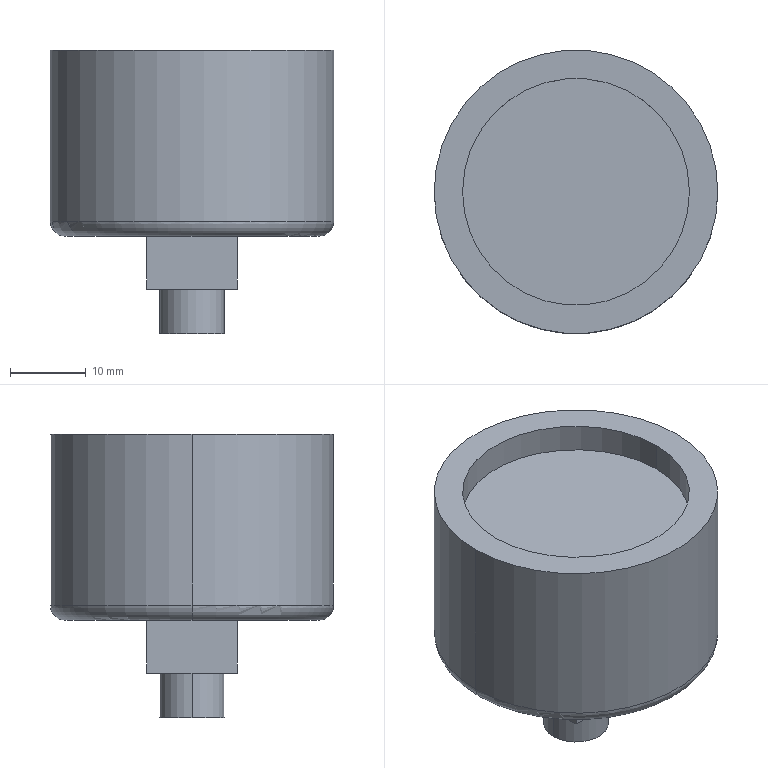Part | STEP file | AR20-G_GAUGE_HI | 1 solid | 17 faces | box 37.5 x 37.5 x 37.5 mm | volume 25733 mm3 | plane 9 | cylinder 6 | torus 2 | commonest cylinder face diameters 8.566 x2 30 x2 37.5 x2
STEP:
#1=CARTESIAN_POINT('',(0.,0.,0.));
#2=DIRECTION('',(0.,0.,1.));
#3=DIRECTION('',(1.,0.,0.));
#4=AXIS2_PLACEMENT_3D('',#1,#2,#3);
#5=CARTESIAN_POINT('',(4.283,0.,27.5));
#6=VERTEX_POINT('',#5);
#7=CARTESIAN_POINT('',(-4.283,0.,27.5));
#8=VERTEX_POINT('',#7);
#9=CARTESIAN_POINT('',(0.,0.,27.5));
#10=DIRECTION('',(0.,0.,1.));
#11=DIRECTION('',(1.,0.,0.));
#12=AXIS2_PLACEMENT_3D('',#9,#10,#11);
#13=CIRCLE('',#12,4.283);
#14=CARTESIAN_POINT('',(0.,0.,27.5));
#15=DIRECTION('',(0.,0.,1.));
#16=DIRECTION('',(1.,0.,0.));
#17=AXIS2_PLACEMENT_3D('',#14,#15,#16);
#18=CYLINDRICAL_SURFACE('',#17,4.283);
#19=CARTESIAN_POINT('',(0.,0.));
#20=DIRECTION('',(1.,0.));
#21=VECTOR('',#20,1.);
#22=LINE('',#19,#21);
#23=(GEOMETRIC_REPRESENTATION_CONTEXT(2)PARAMETRIC_REPRESENTATION_CONTEXT()REPRESENTATION_CONTEXT('',''));
#24=DEFINITIONAL_REPRESENTATION('',(#22),#23);
#25=PCURVE('',#18,#24);
#26=CARTESIAN_POINT('',(0.,4.283,27.5));
#27=DIRECTION('',(0.,0.,1.));
#28=DIRECTION('',(1.,0.,0.));
#29=AXIS2_PLACEMENT_3D('',#26,#27,#28);
#30=PLANE('',#29);
#31=CARTESIAN_POINT('',(0.,-4.283));
#32=DIRECTION('',(1.,0.));
#33=AXIS2_PLACEMENT_2D('',#31,#32);
#34=CIRCLE('',#33,4.283);
#35=(GEOMETRIC_REPRESENTATION_CONTEXT(2)PARAMETRIC_REPRESENTATION_CONTEXT()REPRESENTATION_CONTEXT('',''));
#36=DEFINITIONAL_REPRESENTATION('',(#34),#35);
#37=PCURVE('',#30,#36);
#38=SURFACE_CURVE('',#13,(#25,#37),.PCURVE_S1.);
#39=EDGE_CURVE('',#6,#8,#38,.T.);
#40=ORIENTED_EDGE('',*,*,#39,.T.);
#41=CARTESIAN_POINT('',(-4.283,0.,33.4));
#42=VERTEX_POINT('',#41);
#43=CARTESIAN_POINT('',(-4.283,0.,27.5));
#44=DIRECTION('',(0.,0.,1.));
#45=VECTOR('',#44,1.);
#46=LINE('',#43,#45);
#47=CARTESIAN_POINT('',(3.142,0.));
#48=DIRECTION('',(0.,1.));
#49=VECTOR('',#48,1.);
#50=LINE('',#47,#49);
#51=(GEOMETRIC_REPRESENTATION_CONTEXT(2)PARAMETRIC_REPRESENTATION_CONTEXT()REPRESENTATION_CONTEXT('',''));
#52=DEFINITIONAL_REPRESENTATION('',(#50),#51);
#53=PCURVE('',#18,#52);
#54=CARTESIAN_POINT('',(0.,0.,27.5));
#55=DIRECTION('',(0.,0.,1.));
#56=DIRECTION('',(1.,0.,0.));
#57=AXIS2_PLACEMENT_3D('',#54,#55,#56);
#58=CYLINDRICAL_SURFACE('',#57,4.283);
#59=CARTESIAN_POINT('',(3.142,0.));
#60=DIRECTION('',(0.,1.));
#61=VECTOR('',#60,1.);
#62=LINE('',#59,#61);
#63=(GEOMETRIC_REPRESENTATION_CONTEXT(2)PARAMETRIC_REPRESENTATION_CONTEXT()REPRESENTATION_CONTEXT('',''));
#64=DEFINITIONAL_REPRESENTATION('',(#62),#63);
#65=PCURVE('',#58,#64);
#66=SURFACE_CURVE('',#46,(#53,#65),.PCURVE_S1.);
#67=EDGE_CURVE('',#8,#42,#66,.T.);
#68=ORIENTED_EDGE('',*,*,#67,.T.);
#69=CARTESIAN_POINT('',(4.283,0.,33.4));
#70=VERTEX_POINT('',#69);
#71=CARTESIAN_POINT('',(0.,0.,33.4));
#72=DIRECTION('',(0.,0.,-1.));
#73=DIRECTION('',(1.,0.,0.));
#74=AXIS2_PLACEMENT_3D('',#71,#72,#73);
#75=CIRCLE('',#74,4.283);
#76=CARTESIAN_POINT('',(6.283,5.9));
#77=DIRECTION('',(-1.,0.));
#78=VECTOR('',#77,1.);
#79=LINE('',#76,#78);
#80=(GEOMETRIC_REPRESENTATION_CONTEXT(2)PARAMETRIC_REPRESENTATION_CONTEXT()REPRESENTATION_CONTEXT('',''));
#81=DEFINITIONAL_REPRESENTATION('',(#79),#80);
#82=PCURVE('',#18,#81);
#83=CARTESIAN_POINT('',(6.,-6.,33.4));
#84=DIRECTION('',(0.,0.,1.));
#85=DIRECTION('',(1.,0.,0.));
#86=AXIS2_PLACEMENT_3D('',#83,#84,#85);
#87=PLANE('',#86);
#88=CARTESIAN_POINT('',(-1.717,6.));
#89=CARTESIAN_POINT('',(-1.717,-1.418));
#90=CARTESIAN_POINT('',(-8.142,2.291));
#91=CARTESIAN_POINT('',(-14.566,6.));
#92=CARTESIAN_POINT('',(-8.142,9.709));
#93=CARTESIAN_POINT('',(-1.717,13.418));
#94=CARTESIAN_POINT('',(-1.717,6.));
#95=(BOUNDED_CURVE()B_SPLINE_CURVE(2,(#88,#89,#90,#91,#92,#93,#94),.UNSPECIFIED.,.T.,.F.)B_SPLINE_CURVE_WITH_KNOTS((1,2,2,2,2,1),(-2.094,0.,2.094,4.189,6.283,8.378),.UNSPECIFIED.)CURVE()GEOMETRIC_REPRESENTATION_ITEM()RATIONAL_B_SPLINE_CURVE((1.,0.5,1.,0.5,1.,0.5,1.))REPRESENTATION_ITEM(''));
#96=(GEOMETRIC_REPRESENTATION_CONTEXT(2)PARAMETRIC_REPRESENTATION_CONTEXT()REPRESENTATION_CONTEXT('',''));
#97=DEFINITIONAL_REPRESENTATION('',(#95),#96);
#98=PCURVE('',#87,#97);
#99=SURFACE_CURVE('',#75,(#82,#98),.PCURVE_S1.);
#100=EDGE_CURVE('',#42,#70,#99,.T.);
#101=ORIENTED_EDGE('',*,*,#100,.T.);
#102=CARTESIAN_POINT('',(4.283,0.,27.5));
#103=DIRECTION('',(0.,0.,1.));
#104=VECTOR('',#103,1.);
#105=LINE('',#102,#104);
#106=CARTESIAN_POINT('',(0.,0.));
#107=DIRECTION('',(0.,1.));
#108=VECTOR('',#107,1.);
#109=LINE('',#106,#108);
#110=(GEOMETRIC_REPRESENTATION_CONTEXT(2)PARAMETRIC_REPRESENTATION_CONTEXT()REPRESENTATION_CONTEXT('',''));
#111=DEFINITIONAL_REPRESENTATION('',(#109),#110);
#112=PCURVE('',#18,#111);
#113=CARTESIAN_POINT('',(6.283,0.));
#114=DIRECTION('',(0.,1.));
#115=VECTOR('',#114,1.);
#116=LINE('',#113,#115);
#117=(GEOMETRIC_REPRESENTATION_CONTEXT(2)PARAMETRIC_REPRESENTATION_CONTEXT()REPRESENTATION_CONTEXT('',''));
#118=DEFINITIONAL_REPRESENTATION('',(#116),#117);
#119=PCURVE('',#58,#118);
#120=SURFACE_CURVE('',#105,(#112,#119),.PCURVE_S1.);
#121=EDGE_CURVE('',#6,#70,#120,.T.);
#122=ORIENTED_EDGE('',*,*,#121,.F.);
#123=EDGE_LOOP('',(#40,#68,#101,#122));
#124=FACE_BOUND('',#123,.T.);
#125=ADVANCED_FACE('',(#124),#18,.T.);
#126=CARTESIAN_POINT('',(-15.,0.,65.));
#127=VERTEX_POINT('',#126);
#128=CARTESIAN_POINT('',(-15.,0.,61.2));
#129=VERTEX_POINT('',#128);
#130=CARTESIAN_POINT('',(-15.,0.,61.2));
#131=DIRECTION('',(0.,0.,-1.));
#132=VECTOR('',#131,1.);
#133=LINE('',#130,#132);
#134=CARTESIAN_POINT('',(0.,0.,61.2));
#135=DIRECTION('',(0.,0.,-1.));
#136=DIRECTION('',(-1.,0.,0.));
#137=AXIS2_PLACEMENT_3D('',#134,#135,#136);
#138=CYLINDRICAL_SURFACE('',#137,15.);
#139=CARTESIAN_POINT('',(6.283,0.));
#140=DIRECTION('',(0.,1.));
#141=VECTOR('',#140,1.);
#142=LINE('',#139,#141);
#143=(GEOMETRIC_REPRESENTATION_CONTEXT(2)PARAMETRIC_REPRESENTATION_CONTEXT()REPRESENTATION_CONTEXT('',''));
#144=DEFINITIONAL_REPRESENTATION('',(#142),#143);
#145=PCURVE('',#138,#144);
#146=CARTESIAN_POINT('',(0.,0.,61.2));
#147=DIRECTION('',(0.,0.,-1.));
#148=DIRECTION('',(-1.,0.,0.));
#149=AXIS2_PLACEMENT_3D('',#146,#147,#148);
#150=CYLINDRICAL_SURFACE('',#149,15.);
#151=CARTESIAN_POINT('',(0.,0.));
#152=DIRECTION('',(0.,1.));
#153=VECTOR('',#152,1.);
#154=LINE('',#151,#153);
#155=(GEOMETRIC_REPRESENTATION_CONTEXT(2)PARAMETRIC_REPRESENTATION_CONTEXT()REPRESENTATION_CONTEXT('',''));
#156=DEFINITIONAL_REPRESENTATION('',(#154),#155);
#157=PCURVE('',#150,#156);
#158=SURFACE_CURVE('',#133,(#145,#157),.PCURVE_S1.);
#159=EDGE_CURVE('',#127,#129,#158,.T.);
#160=ORIENTED_EDGE('',*,*,#159,.T.);
#161=CARTESIAN_POINT('',(15.,0.,61.2));
#162=VERTEX_POINT('',#161);
#163=CARTESIAN_POINT('',(0.,0.,61.2));
#164=DIRECTION('',(0.,0.,-1.));
#165=DIRECTION('',(-1.,0.,0.));
#166=AXIS2_PLACEMENT_3D('',#163,#164,#165);
#167=CIRCLE('',#166,15.);
#168=CARTESIAN_POINT('',(0.,0.));
#169=DIRECTION('',(1.,0.));
#170=VECTOR('',#169,1.);
#171=LINE('',#168,#170);
#172=(GEOMETRIC_REPRESENTATION_CONTEXT(2)PARAMETRIC_REPRESENTATION_CONTEXT()REPRESENTATION_CONTEXT('',''));
#173=DEFINITIONAL_REPRESENTATION('',(#171),#172);
#174=PCURVE('',#138,#173);
#175=CARTESIAN_POINT('',(0.,-15.,61.2));
#176=DIRECTION('',(0.,0.,-1.));
#177=DIRECTION('',(-1.,0.,0.));
#178=AXIS2_PLACEMENT_3D('',#175,#176,#177);
#179=PLANE('',#178);
#180=CARTESIAN_POINT('',(0.,15.));
#181=DIRECTION('',(1.,0.));
#182=AXIS2_PLACEMENT_2D('',#180,#181);
#183=CIRCLE('',#182,15.);
#184=(GEOMETRIC_REPRESENTATION_CONTEXT(2)PARAMETRIC_REPRESENTATION_CONTEXT()REPRESENTATION_CONTEXT('',''));
#185=DEFINITIONAL_REPRESENTATION('',(#183),#184);
#186=PCURVE('',#179,#185);
#187=SURFACE_CURVE('',#167,(#174,#186),.PCURVE_S1.);
#188=EDGE_CURVE('',#162,#129,#187,.T.);
#189=ORIENTED_EDGE('',*,*,#188,.F.);
#190=CARTESIAN_POINT('',(15.,0.,65.));
#191=VERTEX_POINT('',#190);
#192=CARTESIAN_POINT('',(15.,0.,61.2));
#193=DIRECTION('',(0.,0.,-1.));
#194=VECTOR('',#193,1.);
#195=LINE('',#192,#194);
#196=CARTESIAN_POINT('',(3.142,0.));
#197=DIRECTION('',(0.,1.));
#198=VECTOR('',#197,1.);
#199=LINE('',#196,#198);
#200=(GEOMETRIC_REPRESENTATION_CONTEXT(2)PARAMETRIC_REPRESENTATION_CONTEXT()REPRESENTATION_CONTEXT('',''));
#201=DEFINITIONAL_REPRESENTATION('',(#199),#200);
#202=PCURVE('',#138,#201);
#203=CARTESIAN_POINT('',(3.142,0.));
#204=DIRECTION('',(0.,1.));
#205=VECTOR('',#204,1.);
#206=LINE('',#203,#205);
#207=(GEOMETRIC_REPRESENTATION_CONTEXT(2)PARAMETRIC_REPRESENTATION_CONTEXT()REPRESENTATION_CONTEXT('',''));
#208=DEFINITIONAL_REPRESENTATION('',(#206),#207);
#209=PCURVE('',#150,#208);
#210=SURFACE_CURVE('',#195,(#202,#209),.PCURVE_S1.);
#211=EDGE_CURVE('',#191,#162,#210,.T.);
#212=ORIENTED_EDGE('',*,*,#211,.F.);
#213=CARTESIAN_POINT('',(0.,0.,65.));
#214=DIRECTION('',(0.,0.,-1.));
#215=DIRECTION('',(-1.,0.,0.));
#216=AXIS2_PLACEMENT_3D('',#213,#214,#215);
#217=CIRCLE('',#216,15.);
#218=CARTESIAN_POINT('',(0.,-3.8));
#219=DIRECTION('',(1.,0.));
#220=VECTOR('',#219,1.);
#221=LINE('',#218,#220);
#222=(GEOMETRIC_REPRESENTATION_CONTEXT(2)PARAMETRIC_REPRESENTATION_CONTEXT()REPRESENTATION_CONTEXT('',''));
#223=DEFINITIONAL_REPRESENTATION('',(#221),#222);
#224=PCURVE('',#138,#223);
#225=CARTESIAN_POINT('',(0.,-18.75,65.));
#226=DIRECTION('',(0.,0.,-1.));
#227=DIRECTION('',(-1.,0.,0.));
#228=AXIS2_PLACEMENT_3D('',#225,#226,#227);
#229=PLANE('',#228);
#230=CARTESIAN_POINT('',(0.,18.75));
#231=DIRECTION('',(1.,0.));
#232=AXIS2_PLACEMENT_2D('',#230,#231);
#233=CIRCLE('',#232,15.);
#234=(GEOMETRIC_REPRESENTATION_CONTEXT(2)PARAMETRIC_REPRESENTATION_CONTEXT()REPRESENTATION_CONTEXT('',''));
#235=DEFINITIONAL_REPRESENTATION('',(#233),#234);
#236=PCURVE('',#229,#235);
#237=SURFACE_CURVE('',#217,(#224,#236),.PCURVE_S1.);
#238=EDGE_CURVE('',#191,#127,#237,.T.);
#239=ORIENTED_EDGE('',*,*,#238,.T.);
#240=EDGE_LOOP('',(#160,#189,#212,#239));
#241=FACE_BOUND('',#240,.F.);
#242=ADVANCED_FACE('',(#241),#138,.F.);
#243=CARTESIAN_POINT('',(-18.75,0.,65.));
#244=VERTEX_POINT('',#243);
#245=CARTESIAN_POINT('',(18.75,0.,65.));
#246=VERTEX_POINT('',#245);
#247=CARTESIAN_POINT('',(0.,0.,65.));
#248=DIRECTION('',(0.,0.,-1.));
#249=DIRECTION('',(-1.,0.,0.));
#250=AXIS2_PLACEMENT_3D('',#247,#248,#249);
#251=CIRCLE('',#250,18.75);
#252=CARTESIAN_POINT('',(0.,0.,61.2));
#253=DIRECTION('',(0.,0.,-1.));
#254=DIRECTION('',(-1.,0.,0.));
#255=AXIS2_PLACEMENT_3D('',#252,#253,#254);
#256=CYLINDRICAL_SURFACE('',#255,18.75);
#257=CARTESIAN_POINT('',(0.,-3.8));
#258=DIRECTION('',(1.,0.));
#259=VECTOR('',#258,1.);
#260=LINE('',#257,#259);
#261=(GEOMETRIC_REPRESENTATION_CONTEXT(2)PARAMETRIC_REPRESENTATION_CONTEXT()REPRESENTATION_CONTEXT('',''));
#262=DEFINITIONAL_REPRESENTATION('',(#260),#261);
#263=PCURVE('',#256,#262);
#264=CARTESIAN_POINT('',(0.,18.75));
#265=DIRECTION('',(1.,0.));
#266=AXIS2_PLACEMENT_2D('',#264,#265);
#267=CIRCLE('',#266,18.75);
#268=(GEOMETRIC_REPRESENTATION_CONTEXT(2)PARAMETRIC_REPRESENTATION_CONTEXT()REPRESENTATION_CONTEXT('',''));
#269=DEFINITIONAL_REPRESENTATION('',(#267),#268);
#270=PCURVE('',#229,#269);
#271=SURFACE_CURVE('',#251,(#263,#270),.PCURVE_S1.);
#272=EDGE_CURVE('',#244,#246,#271,.T.);
#273=ORIENTED_EDGE('',*,*,#272,.T.);
#274=CARTESIAN_POINT('',(18.75,0.,42.4));
#275=VERTEX_POINT('',#274);
#276=CARTESIAN_POINT('',(18.75,0.,61.2));
#277=DIRECTION('',(0.,0.,-1.));
#278=VECTOR('',#277,1.);
#279=LINE('',#276,#278);
#280=CARTESIAN_POINT('',(3.142,0.));
#281=DIRECTION('',(0.,1.));
#282=VECTOR('',#281,1.);
#283=LINE('',#280,#282);
#284=(GEOMETRIC_REPRESENTATION_CONTEXT(2)PARAMETRIC_REPRESENTATION_CONTEXT()REPRESENTATION_CONTEXT('',''));
#285=DEFINITIONAL_REPRESENTATION('',(#283),#284);
#286=PCURVE('',#256,#285);
#287=CARTESIAN_POINT('',(0.,0.,61.2));
#288=DIRECTION('',(0.,0.,-1.));
#289=DIRECTION('',(-1.,0.,0.));
#290=AXIS2_PLACEMENT_3D('',#287,#288,#289);
#291=CYLINDRICAL_SURFACE('',#290,18.75);
#292=CARTESIAN_POINT('',(3.142,0.));
#293=DIRECTION('',(0.,1.));
#294=VECTOR('',#293,1.);
#295=LINE('',#292,#294);
#296=(GEOMETRIC_REPRESENTATION_CONTEXT(2)PARAMETRIC_REPRESENTATION_CONTEXT()REPRESENTATION_CONTEXT('',''));
#297=DEFINITIONAL_REPRESENTATION('',(#295),#296);
#298=PCURVE('',#291,#297);
#299=SURFACE_CURVE('',#279,(#286,#298),.PCURVE_S1.);
#300=EDGE_CURVE('',#246,#275,#299,.T.);
#301=ORIENTED_EDGE('',*,*,#300,.T.);
#302=CARTESIAN_POINT('',(-18.75,0.,42.4));
#303=VERTEX_POINT('',#302);
#304=CARTESIAN_POINT('',(0.,0.,42.4));
#305=DIRECTION('',(0.,0.,-1.));
#306=DIRECTION('',(-1.,0.,0.));
#307=AXIS2_PLACEMENT_3D('',#304,#305,#306);
#308=CIRCLE('',#307,18.75);
#309=CARTESIAN_POINT('',(0.,18.8));
#310=DIRECTION('',(1.,0.));
#311=VECTOR('',#310,1.);
#312=LINE('',#309,#311);
#313=(GEOMETRIC_REPRESENTATION_CONTEXT(2)PARAMETRIC_REPRESENTATION_CONTEXT()REPRESENTATION_CONTEXT('',''));
#314=DEFINITIONAL_REPRESENTATION('',(#312),#313);
#315=PCURVE('',#256,#314);
#316=CARTESIAN_POINT('',(0.,0.,42.4));
#317=DIRECTION('',(0.,0.,-1.));
#318=DIRECTION('',(-1.,0.,0.));
#319=AXIS2_PLACEMENT_3D('',#316,#317,#318);
#320=TOROIDAL_SURFACE('',#319,16.75,2.);
#321=CARTESIAN_POINT('',(0.,0.));
#322=DIRECTION('',(1.,0.));
#323=VECTOR('',#322,1.);
#324=LINE('',#321,#323);
#325=(GEOMETRIC_REPRESENTATION_CONTEXT(2)PARAMETRIC_REPRESENTATION_CONTEXT()REPRESENTATION_CONTEXT('',''));
#326=DEFINITIONAL_REPRESENTATION('',(#324),#325);
#327=PCURVE('',#320,#326);
#328=SURFACE_CURVE('',#308,(#315,#327),.PCURVE_S1.);
#329=EDGE_CURVE('',#303,#275,#328,.T.);
#330=ORIENTED_EDGE('',*,*,#329,.F.);
#331=CARTESIAN_POINT('',(-18.75,0.,61.2));
#332=DIRECTION('',(0.,0.,-1.));
#333=VECTOR('',#332,1.);
#334=LINE('',#331,#333);
#335=CARTESIAN_POINT('',(0.,0.));
#336=DIRECTION('',(0.,1.));
#337=VECTOR('',#336,1.);
#338=LINE('',#335,#337);
#339=(GEOMETRIC_REPRESENTATION_CONTEXT(2)PARAMETRIC_REPRESENTATION_CONTEXT()REPRESENTATION_CONTEXT('',''));
#340=DEFINITIONAL_REPRESENTATION('',(#338),#339);
#341=PCURVE('',#256,#340);
#342=CARTESIAN_POINT('',(6.283,0.));
#343=DIRECTION('',(0.,1.));
#344=VECTOR('',#343,1.);
#345=LINE('',#342,#344);
#346=(GEOMETRIC_REPRESENTATION_CONTEXT(2)PARAMETRIC_REPRESENTATION_CONTEXT()REPRESENTATION_CONTEXT('',''));
#347=DEFINITIONAL_REPRESENTATION('',(#345),#346);
#348=PCURVE('',#291,#347);
#349=SURFACE_CURVE('',#334,(#341,#348),.PCURVE_S1.);
#350=EDGE_CURVE('',#244,#303,#349,.T.);
#351=ORIENTED_EDGE('',*,*,#350,.F.);
#352=EDGE_LOOP('',(#273,#301,#330,#351));
#353=FACE_BOUND('',#352,.T.);
#354=ADVANCED_FACE('',(#353),#256,.T.);
#355=ORIENTED_EDGE('',*,*,#329,.T.);
#356=CARTESIAN_POINT('',(16.75,0.,40.4));
#357=VERTEX_POINT('',#356);
#358=CARTESIAN_POINT('',(16.75,0.,42.4));
#359=DIRECTION('',(0.,1.,0.));
#360=DIRECTION('',(-1.,0.,0.));
#361=AXIS2_PLACEMENT_3D('',#358,#359,#360);
#362=CIRCLE('',#361,2.);
#363=CARTESIAN_POINT('',(3.142,-3.142));
#364=DIRECTION('',(0.,1.));
#365=VECTOR('',#364,1.);
#366=LINE('',#363,#365);
#367=(GEOMETRIC_REPRESENTATION_CONTEXT(2)PARAMETRIC_REPRESENTATION_CONTEXT()REPRESENTATION_CONTEXT('',''));
#368=DEFINITIONAL_REPRESENTATION('',(#366),#367);
#369=PCURVE('',#320,#368);
#370=CARTESIAN_POINT('',(0.,0.,42.4));
#371=DIRECTION('',(0.,0.,-1.));
#372=DIRECTION('',(-1.,0.,0.));
#373=AXIS2_PLACEMENT_3D('',#370,#371,#372);
#374=TOROIDAL_SURFACE('',#373,16.75,2.);
#375=CARTESIAN_POINT('',(3.142,-3.142));
#376=DIRECTION('',(0.,1.));
#377=VECTOR('',#376,1.);
#378=LINE('',#375,#377);
#379=(GEOMETRIC_REPRESENTATION_CONTEXT(2)PARAMETRIC_REPRESENTATION_CONTEXT()REPRESENTATION_CONTEXT('',''));
#380=DEFINITIONAL_REPRESENTATION('',(#378),#379);
#381=PCURVE('',#374,#380);
#382=SURFACE_CURVE('',#362,(#369,#381),.PCURVE_S1.);
#383=EDGE_CURVE('',#275,#357,#382,.T.);
#384=ORIENTED_EDGE('',*,*,#383,.T.);
#385=CARTESIAN_POINT('',(-16.75,0.,40.4));
#386=VERTEX_POINT('',#385);
#387=CARTESIAN_POINT('',(0.,0.,40.4));
#388=DIRECTION('',(0.,0.,-1.));
#389=DIRECTION('',(-1.,0.,0.));
#390=AXIS2_PLACEMENT_3D('',#387,#388,#389);
#391=CIRCLE('',#390,16.75);
#392=CARTESIAN_POINT('',(0.,1.571));
#393=DIRECTION('',(1.,0.));
#394=VECTOR('',#393,1.);
#395=LINE('',#392,#394);
#396=(GEOMETRIC_REPRESENTATION_CONTEXT(2)PARAMETRIC_REPRESENTATION_CONTEXT()REPRESENTATION_CONTEXT('',''));
#397=DEFINITIONAL_REPRESENTATION('',(#395),#396);
#398=PCURVE('',#320,#397);
#399=CARTESIAN_POINT('',(0.,0.,40.4));
#400=DIRECTION('',(0.,0.,1.));
#401=DIRECTION('',(1.,0.,0.));
#402=AXIS2_PLACEMENT_3D('',#399,#400,#401);
#403=PLANE('',#402);
#404=CARTESIAN_POINT('',(-16.75,0.));
#405=CARTESIAN_POINT('',(-16.75,29.012));
#406=CARTESIAN_POINT('',(8.375,14.506));
#407=CARTESIAN_POINT('',(33.5,0.));
#408=CARTESIAN_POINT('',(8.375,-14.506));
#409=CARTESIAN_POINT('',(-16.75,-29.012));
#410=CARTESIAN_POINT('',(-16.75,0.));
#411=(BOUNDED_CURVE()B_SPLINE_CURVE(2,(#404,#405,#406,#407,#408,#409,#410),.UNSPECIFIED.,.T.,.F.)B_SPLINE_CURVE_WITH_KNOTS((1,2,2,2,2,1),(-2.094,0.,2.094,4.189,6.283,8.378),.UNSPECIFIED.)CURVE()GEOMETRIC_REPRESENTATION_ITEM()RATIONAL_B_SPLINE_CURVE((1.,0.5,1.,0.5,1.,0.5,1.))REPRESENTATION_ITEM(''));
#412=(GEOMETRIC_REPRESENTATION_CONTEXT(2)PARAMETRIC_REPRESENTATION_CONTEXT()REPRESENTATION_CONTEXT('',''));
#413=DEFINITIONAL_REPRESENTATION('',(#411),#412);
#414=PCURVE('',#403,#413);
#415=SURFACE_CURVE('',#391,(#398,#414),.PCURVE_S1.);
#416=EDGE_CURVE('',#386,#357,#415,.T.);
#417=ORIENTED_EDGE('',*,*,#416,.F.);
#418=CARTESIAN_POINT('',(-16.75,0.,42.4));
#419=DIRECTION('',(0.,-1.,0.));
#420=DIRECTION('',(0.,0.,-1.));
#421=AXIS2_PLACEMENT_3D('',#418,#419,#420);
#422=CIRCLE('',#421,2.);
#423=CARTESIAN_POINT('',(0.,-4.712));
#424=DIRECTION('',(0.,1.));
#425=VECTOR('',#424,1.);
#426=LINE('',#423,#425);
#427=(GEOMETRIC_REPRESENTATION_CONTEXT(2)PARAMETRIC_REPRESENTATION_CONTEXT()REPRESENTATION_CONTEXT('',''));
#428=DEFINITIONAL_REPRESENTATION('',(#426),#427);
#429=PCURVE('',#320,#428);
#430=CARTESIAN_POINT('',(6.283,-4.712));
#431=DIRECTION('',(0.,1.));
#432=VECTOR('',#431,1.);
#433=LINE('',#430,#432);
#434=(GEOMETRIC_REPRESENTATION_CONTEXT(2)PARAMETRIC_REPRESENTATION_CONTEXT()REPRESENTATION_CONTEXT('',''));
#435=DEFINITIONAL_REPRESENTATION('',(#433),#434);
#436=PCURVE('',#374,#435);
#437=SURFACE_CURVE('',#422,(#429,#436),.PCURVE_S1.);
#438=EDGE_CURVE('',#303,#386,#437,.T.);
#439=ORIENTED_EDGE('',*,*,#438,.F.);
#440=EDGE_LOOP('',(#355,#384,#417,#439));
#441=FACE_BOUND('',#440,.T.);
#442=ADVANCED_FACE('',(#441),#320,.T.);
#443=CARTESIAN_POINT('',(6.,-6.,33.4));
#444=VERTEX_POINT('',#443);
#445=CARTESIAN_POINT('',(-6.,-6.,33.4));
#446=VERTEX_POINT('',#445);
#447=CARTESIAN_POINT('',(6.,-6.,33.4));
#448=DIRECTION('',(-1.,0.,0.));
#449=VECTOR('',#448,1.);
#450=LINE('',#447,#449);
#451=CARTESIAN_POINT('',(0.,0.));
#452=DIRECTION('',(-1.,0.));
#453=VECTOR('',#452,1.);
#454=LINE('',#451,#453);
#455=(GEOMETRIC_REPRESENTATION_CONTEXT(2)PARAMETRIC_REPRESENTATION_CONTEXT()REPRESENTATION_CONTEXT('',''));
#456=DEFINITIONAL_REPRESENTATION('',(#454),#455);
#457=PCURVE('',#87,#456);
#458=CARTESIAN_POINT('',(6.,-6.,40.4));
#459=DIRECTION('',(0.,1.,0.));
#460=DIRECTION('',(0.,0.,1.));
#461=AXIS2_PLACEMENT_3D('',#458,#459,#460);
#462=PLANE('',#461);
#463=CARTESIAN_POINT('',(-7.,0.));
#464=DIRECTION('',(0.,-1.));
#465=VECTOR('',#464,1.);
#466=LINE('',#463,#465);
#467=(GEOMETRIC_REPRESENTATION_CONTEXT(2)PARAMETRIC_REPRESENTATION_CONTEXT()REPRESENTATION_CONTEXT('',''));
#468=DEFINITIONAL_REPRESENTATION('',(#466),#467);
#469=PCURVE('',#462,#468);
#470=SURFACE_CURVE('',#450,(#457,#469),.PCURVE_S1.);
#471=EDGE_CURVE('',#444,#446,#470,.T.);
#472=ORIENTED_EDGE('',*,*,#471,.T.);
#473=CARTESIAN_POINT('',(-6.,6.,33.4));
#474=VERTEX_POINT('',#473);
#475=CARTESIAN_POINT('',(-6.,-6.,33.4));
#476=DIRECTION('',(0.,1.,0.));
#477=VECTOR('',#476,1.);
#478=LINE('',#475,#477);
#479=CARTESIAN_POINT('',(-12.,0.));
#480=DIRECTION('',(0.,1.));
#481=VECTOR('',#480,1.);
#482=LINE('',#479,#481);
#483=(GEOMETRIC_REPRESENTATION_CONTEXT(2)PARAMETRIC_REPRESENTATION_CONTEXT()REPRESENTATION_CONTEXT('',''));
#484=DEFINITIONAL_REPRESENTATION('',(#482),#483);
#485=PCURVE('',#87,#484);
#486=CARTESIAN_POINT('',(-6.,0.,0.));
#487=DIRECTION('',(1.,0.,0.));
#488=DIRECTION('',(0.,0.,-1.));
#489=AXIS2_PLACEMENT_3D('',#486,#487,#488);
#490=PLANE('',#489);
#491=CARTESIAN_POINT('',(-33.4,-6.));
#492=DIRECTION('',(0.,1.));
#493=VECTOR('',#492,1.);
#494=LINE('',#491,#493);
#495=(GEOMETRIC_REPRESENTATION_CONTEXT(2)PARAMETRIC_REPRESENTATION_CONTEXT()REPRESENTATION_CONTEXT('',''));
#496=DEFINITIONAL_REPRESENTATION('',(#494),#495);
#497=PCURVE('',#490,#496);
#498=SURFACE_CURVE('',#478,(#485,#497),.PCURVE_S1.);
#499=EDGE_CURVE('',#446,#474,#498,.T.);
#500=ORIENTED_EDGE('',*,*,#499,.T.);
#501=CARTESIAN_POINT('',(6.,6.,33.4));
#502=VERTEX_POINT('',#501);
#503=CARTESIAN_POINT('',(6.,6.,33.4));
#504=DIRECTION('',(-1.,0.,0.));
#505=VECTOR('',#504,1.);
#506=LINE('',#503,#505);
#507=CARTESIAN_POINT('',(0.,12.));
#508=DIRECTION('',(-1.,0.));
#509=VECTOR('',#508,1.);
#510=LINE('',#507,#509);
#511=(GEOMETRIC_REPRESENTATION_CONTEXT(2)PARAMETRIC_REPRESENTATION_CONTEXT()REPRESENTATION_CONTEXT('',''));
#512=DEFINITIONAL_REPRESENTATION('',(#510),#511);
#513=PCURVE('',#87,#512);
#514=CARTESIAN_POINT('',(6.,6.,33.4));
#515=DIRECTION('',(0.,-1.,0.));
#516=DIRECTION('',(0.,0.,-1.));
#517=AXIS2_PLACEMENT_3D('',#514,#515,#516);
#518=PLANE('',#517);
#519=CARTESIAN_POINT('',(0.,0.));
#520=DIRECTION('',(0.,-1.));
#521=VECTOR('',#520,1.);
#522=LINE('',#519,#521);
#523=(GEOMETRIC_REPRESENTATION_CONTEXT(2)PARAMETRIC_REPRESENTATION_CONTEXT()REPRESENTATION_CONTEXT('',''));
#524=DEFINITIONAL_REPRESENTATION('',(#522),#523);
#525=PCURVE('',#518,#524);
#526=SURFACE_CURVE('',#506,(#513,#525),.PCURVE_S1.);
#527=EDGE_CURVE('',#502,#474,#526,.T.);
#528=ORIENTED_EDGE('',*,*,#527,.F.);
#529=CARTESIAN_POINT('',(6.,-6.,33.4));
#530=DIRECTION('',(0.,1.,0.));
#531=VECTOR('',#530,1.);
#532=LINE('',#529,#531);
#533=CARTESIAN_POINT('',(0.,0.));
#534=DIRECTION('',(0.,1.));
#535=VECTOR('',#534,1.);
#536=LINE('',#533,#535);
#537=(GEOMETRIC_REPRESENTATION_CONTEXT(2)PARAMETRIC_REPRESENTATION_CONTEXT()REPRESENTATION_CONTEXT('',''));
#538=DEFINITIONAL_REPRESENTATION('',(#536),#537);
#539=PCURVE('',#87,#538);
#540=CARTESIAN_POINT('',(6.,0.,0.));
#541=DIRECTION('',(1.,0.,0.));
#542=DIRECTION('',(0.,0.,-1.));
#543=AXIS2_PLACEMENT_3D('',#540,#541,#542);
#544=PLANE('',#543);
#545=CARTESIAN_POINT('',(-33.4,-6.));
#546=DIRECTION('',(0.,1.));
#547=VECTOR('',#546,1.);
#548=LINE('',#545,#547);
#549=(GEOMETRIC_REPRESENTATION_CONTEXT(2)PARAMETRIC_REPRESENTATION_CONTEXT()REPRESENTATION_CONTEXT('',''));
#550=DEFINITIONAL_REPRESENTATION('',(#548),#549);
#551=PCURVE('',#544,#550);
#552=SURFACE_CURVE('',#532,(#539,#551),.PCURVE_S1.);
#553=EDGE_CURVE('',#444,#502,#552,.T.);
#554=ORIENTED_EDGE('',*,*,#553,.F.);
#555=EDGE_LOOP('',(#472,#500,#528,#554));
#556=FACE_BOUND('',#555,.T.);
#557=CARTESIAN_POINT('',(0.,0.,33.4));
#558=DIRECTION('',(0.,0.,-1.));
#559=DIRECTION('',(1.,0.,0.));
#560=AXIS2_PLACEMENT_3D('',#557,#558,#559);
#561=CIRCLE('',#560,4.283);
#562=CARTESIAN_POINT('',(-1.717,6.));
#563=CARTESIAN_POINT('',(-1.717,-1.418));
#564=CARTESIAN_POINT('',(-8.142,2.291));
#565=CARTESIAN_POINT('',(-14.566,6.));
#566=CARTESIAN_POINT('',(-8.142,9.709));
#567=CARTESIAN_POINT('',(-1.717,13.418));
#568=CARTESIAN_POINT('',(-1.717,6.));
#569=(BOUNDED_CURVE()B_SPLINE_CURVE(2,(#562,#563,#564,#565,#566,#567,#568),.UNSPECIFIED.,.T.,.F.)B_SPLINE_CURVE_WITH_KNOTS((1,2,2,2,2,1),(-2.094,0.,2.094,4.189,6.283,8.378),.UNSPECIFIED.)CURVE()GEOMETRIC_REPRESENTATION_ITEM()RATIONAL_B_SPLINE_CURVE((1.,0.5,1.,0.5,1.,0.5,1.))REPRESENTATION_ITEM(''));
#570=(GEOMETRIC_REPRESENTATION_CONTEXT(2)PARAMETRIC_REPRESENTATION_CONTEXT()REPRESENTATION_CONTEXT('',''));
#571=DEFINITIONAL_REPRESENTATION('',(#569),#570);
#572=PCURVE('',#87,#571);
#573=CARTESIAN_POINT('',(6.283,5.9));
#574=DIRECTION('',(-1.,0.));
#575=VECTOR('',#574,1.);
#576=LINE('',#573,#575);
#577=(GEOMETRIC_REPRESENTATION_CONTEXT(2)PARAMETRIC_REPRESENTATION_CONTEXT()REPRESENTATION_CONTEXT('',''));
#578=DEFINITIONAL_REPRESENTATION('',(#576),#577);
#579=PCURVE('',#58,#578);
#580=SURFACE_CURVE('',#561,(#572,#579),.PCURVE_S1.);
#581=EDGE_CURVE('',#70,#42,#580,.T.);
#582=ORIENTED_EDGE('',*,*,#581,.F.);
#583=ORIENTED_EDGE('',*,*,#100,.F.);
#584=EDGE_LOOP('',(#582,#583));
#585=FACE_BOUND('',#584,.T.);
#586=ADVANCED_FACE('',(#556,#585),#87,.F.);
#587=CARTESIAN_POINT('',(6.,-6.,40.4));
#588=VERTEX_POINT('',#587);
#589=CARTESIAN_POINT('',(-6.,-6.,40.4));
#590=VERTEX_POINT('',#589);
#591=CARTESIAN_POINT('',(6.,-6.,40.4));
#592=DIRECTION('',(-1.,0.,0.));
#593=VECTOR('',#592,1.);
#594=LINE('',#591,#593);
#595=CARTESIAN_POINT('',(6.,-6.));
#596=DIRECTION('',(-1.,0.));
#597=VECTOR('',#596,1.);
#598=LINE('',#595,#597);
#599=(GEOMETRIC_REPRESENTATION_CONTEXT(2)PARAMETRIC_REPRESENTATION_CONTEXT()REPRESENTATION_CONTEXT('',''));
#600=DEFINITIONAL_REPRESENTATION('',(#598),#599);
#601=PCURVE('',#403,#600);
#602=CARTESIAN_POINT('',(0.,0.));
#603=DIRECTION('',(0.,-1.));
#604=VECTOR('',#603,1.);
#605=LINE('',#602,#604);
#606=(GEOMETRIC_REPRESENTATION_CONTEXT(2)PARAMETRIC_REPRESENTATION_CONTEXT()REPRESENTATION_CONTEXT('',''));
#607=DEFINITIONAL_REPRESENTATION('',(#605),#606);
#608=PCURVE('',#462,#607);
#609=SURFACE_CURVE('',#594,(#601,#608),.PCURVE_S1.);
#610=EDGE_CURVE('',#588,#590,#609,.T.);
#611=ORIENTED_EDGE('',*,*,#610,.F.);
#612=CARTESIAN_POINT('',(6.,6.,40.4));
#613=VERTEX_POINT('',#612);
#614=CARTESIAN_POINT('',(6.,6.,40.4));
#615=DIRECTION('',(0.,-1.,0.));
#616=VECTOR('',#615,1.);
#617=LINE('',#614,#616);
#618=CARTESIAN_POINT('',(6.,6.));
#619=DIRECTION('',(0.,-1.));
#620=VECTOR('',#619,1.);
#621=LINE('',#618,#620);
#622=(GEOMETRIC_REPRESENTATION_CONTEXT(2)PARAMETRIC_REPRESENTATION_CONTEXT()REPRESENTATION_CONTEXT('',''));
#623=DEFINITIONAL_REPRESENTATION('',(#621),#622);
#624=PCURVE('',#403,#623);
#625=CARTESIAN_POINT('',(-40.4,6.));
#626=DIRECTION('',(0.,-1.));
#627=VECTOR('',#626,1.);
#628=LINE('',#625,#627);
#629=(GEOMETRIC_REPRESENTATION_CONTEXT(2)PARAMETRIC_REPRESENTATION_CONTEXT()REPRESENTATION_CONTEXT('',''));
#630=DEFINITIONAL_REPRESENTATION('',(#628),#629);
#631=PCURVE('',#544,#630);
#632=SURFACE_CURVE('',#617,(#624,#631),.PCURVE_S1.);
#633=EDGE_CURVE('',#613,#588,#632,.T.);
#634=ORIENTED_EDGE('',*,*,#633,.F.);
#635=CARTESIAN_POINT('',(-6.,6.,40.4));
#636=VERTEX_POINT('',#635);
#637=CARTESIAN_POINT('',(6.,6.,40.4));
#638=DIRECTION('',(-1.,0.,0.));
#639=VECTOR('',#638,1.);
#640=LINE('',#637,#639);
#641=CARTESIAN_POINT('',(6.,6.));
#642=DIRECTION('',(-1.,0.));
#643=VECTOR('',#642,1.);
#644=LINE('',#641,#643);
#645=(GEOMETRIC_REPRESENTATION_CONTEXT(2)PARAMETRIC_REPRESENTATION_CONTEXT()REPRESENTATION_CONTEXT('',''));
#646=DEFINITIONAL_REPRESENTATION('',(#644),#645);
#647=PCURVE('',#403,#646);
#648=CARTESIAN_POINT('',(-7.,0.));
#649=DIRECTION('',(0.,-1.));
#650=VECTOR('',#649,1.);
#651=LINE('',#648,#650);
#652=(GEOMETRIC_REPRESENTATION_CONTEXT(2)PARAMETRIC_REPRESENTATION_CONTEXT()REPRESENTATION_CONTEXT('',''));
#653=DEFINITIONAL_REPRESENTATION('',(#651),#652);
#654=PCURVE('',#518,#653);
#655=SURFACE_CURVE('',#640,(#647,#654),.PCURVE_S1.);
#656=EDGE_CURVE('',#613,#636,#655,.T.);
#657=ORIENTED_EDGE('',*,*,#656,.T.);
#658=CARTESIAN_POINT('',(-6.,6.,40.4));
#659=DIRECTION('',(0.,-1.,0.));
#660=VECTOR('',#659,1.);
#661=LINE('',#658,#660);
#662=CARTESIAN_POINT('',(-6.,6.));
#663=DIRECTION('',(0.,-1.));
#664=VECTOR('',#663,1.);
#665=LINE('',#662,#664);
#666=(GEOMETRIC_REPRESENTATION_CONTEXT(2)PARAMETRIC_REPRESENTATION_CONTEXT()REPRESENTATION_CONTEXT('',''));
#667=DEFINITIONAL_REPRESENTATION('',(#665),#666);
#668=PCURVE('',#403,#667);
#669=CARTESIAN_POINT('',(-40.4,6.));
#670=DIRECTION('',(0.,-1.));
#671=VECTOR('',#670,1.);
#672=LINE('',#669,#671);
#673=(GEOMETRIC_REPRESENTATION_CONTEXT(2)PARAMETRIC_REPRESENTATION_CONTEXT()REPRESENTATION_CONTEXT('',''));
#674=DEFINITIONAL_REPRESENTATION('',(#672),#673);
#675=PCURVE('',#490,#674);
#676=SURFACE_CURVE('',#661,(#668,#675),.PCURVE_S1.);
#677=EDGE_CURVE('',#636,#590,#676,.T.);
#678=ORIENTED_EDGE('',*,*,#677,.T.);
#679=EDGE_LOOP('',(#611,#634,#657,#678));
#680=FACE_BOUND('',#679,.T.);
#681=ORIENTED_EDGE('',*,*,#416,.T.);
#682=CARTESIAN_POINT('',(0.,0.,40.4));
#683=DIRECTION('',(0.,0.,-1.));
#684=DIRECTION('',(-1.,0.,0.));
#685=AXIS2_PLACEMENT_3D('',#682,#683,#684);
#686=CIRCLE('',#685,16.75);
#687=CARTESIAN_POINT('',(-16.75,0.));
#688=CARTESIAN_POINT('',(-16.75,29.012));
#689=CARTESIAN_POINT('',(8.375,14.506));
#690=CARTESIAN_POINT('',(33.5,0.));
#691=CARTESIAN_POINT('',(8.375,-14.506));
#692=CARTESIAN_POINT('',(-16.75,-29.012));
#693=CARTESIAN_POINT('',(-16.75,0.));
#694=(BOUNDED_CURVE()B_SPLINE_CURVE(2,(#687,#688,#689,#690,#691,#692,#693),.UNSPECIFIED.,.T.,.F.)B_SPLINE_CURVE_WITH_KNOTS((1,2,2,2,2,1),(-2.094,0.,2.094,4.189,6.283,8.378),.UNSPECIFIED.)CURVE()GEOMETRIC_REPRESENTATION_ITEM()RATIONAL_B_SPLINE_CURVE((1.,0.5,1.,0.5,1.,0.5,1.))REPRESENTATION_ITEM(''));
#695=(GEOMETRIC_REPRESENTATION_CONTEXT(2)PARAMETRIC_REPRESENTATION_CONTEXT()REPRESENTATION_CONTEXT('',''));
#696=DEFINITIONAL_REPRESENTATION('',(#694),#695);
#697=PCURVE('',#403,#696);
#698=CARTESIAN_POINT('',(0.,1.571));
#699=DIRECTION('',(1.,0.));
#700=VECTOR('',#699,1.);
#701=LINE('',#698,#700);
#702=(GEOMETRIC_REPRESENTATION_CONTEXT(2)PARAMETRIC_REPRESENTATION_CONTEXT()REPRESENTATION_CONTEXT('',''));
#703=DEFINITIONAL_REPRESENTATION('',(#701),#702);
#704=PCURVE('',#374,#703);
#705=SURFACE_CURVE('',#686,(#697,#704),.PCURVE_S1.);
#706=EDGE_CURVE('',#357,#386,#705,.T.);
#707=ORIENTED_EDGE('',*,*,#706,.T.);
#708=EDGE_LOOP('',(#681,#707));
#709=FACE_BOUND('',#708,.T.);
#710=ADVANCED_FACE('',(#680,#709),#403,.F.);
#711=ORIENTED_EDGE('',*,*,#383,.F.);
#712=CARTESIAN_POINT('',(0.,0.,42.4));
#713=DIRECTION('',(0.,0.,-1.));
#714=DIRECTION('',(-1.,0.,0.));
#715=AXIS2_PLACEMENT_3D('',#712,#713,#714);
#716=CIRCLE('',#715,18.75);
#717=CARTESIAN_POINT('',(0.,0.));
#718=DIRECTION('',(1.,0.));
#719=VECTOR('',#718,1.);
#720=LINE('',#717,#719);
#721=(GEOMETRIC_REPRESENTATION_CONTEXT(2)PARAMETRIC_REPRESENTATION_CONTEXT()REPRESENTATION_CONTEXT('',''));
#722=DEFINITIONAL_REPRESENTATION('',(#720),#721);
#723=PCURVE('',#374,#722);
#724=CARTESIAN_POINT('',(0.,18.8));
#725=DIRECTION('',(1.,0.));
#726=VECTOR('',#725,1.);
#727=LINE('',#724,#726);
#728=(GEOMETRIC_REPRESENTATION_CONTEXT(2)PARAMETRIC_REPRESENTATION_CONTEXT()REPRESENTATION_CONTEXT('',''));
#729=DEFINITIONAL_REPRESENTATION('',(#727),#728);
#730=PCURVE('',#291,#729);
#731=SURFACE_CURVE('',#716,(#723,#730),.PCURVE_S1.);
#732=EDGE_CURVE('',#275,#303,#731,.T.);
#733=ORIENTED_EDGE('',*,*,#732,.T.);
#734=ORIENTED_EDGE('',*,*,#438,.T.);
#735=ORIENTED_EDGE('',*,*,#706,.F.);
#736=EDGE_LOOP('',(#711,#733,#734,#735));
#737=FACE_BOUND('',#736,.T.);
#738=ADVANCED_FACE('',(#737),#374,.T.);
#739=ORIENTED_EDGE('',*,*,#300,.F.);
#740=CARTESIAN_POINT('',(0.,0.,65.));
#741=DIRECTION('',(0.,0.,-1.));
#742=DIRECTION('',(-1.,0.,0.));
#743=AXIS2_PLACEMENT_3D('',#740,#741,#742);
#744=CIRCLE('',#743,18.75);
#745=CARTESIAN_POINT('',(0.,-3.8));
#746=DIRECTION('',(1.,0.));
#747=VECTOR('',#746,1.);
#748=LINE('',#745,#747);
#749=(GEOMETRIC_REPRESENTATION_CONTEXT(2)PARAMETRIC_REPRESENTATION_CONTEXT()REPRESENTATION_CONTEXT('',''));
#750=DEFINITIONAL_REPRESENTATION('',(#748),#749);
#751=PCURVE('',#291,#750);
#752=CARTESIAN_POINT('',(0.,18.75));
#753=DIRECTION('',(1.,0.));
#754=AXIS2_PLACEMENT_2D('',#752,#753);
#755=CIRCLE('',#754,18.75);
#756=(GEOMETRIC_REPRESENTATION_CONTEXT(2)PARAMETRIC_REPRESENTATION_CONTEXT()REPRESENTATION_CONTEXT('',''));
#757=DEFINITIONAL_REPRESENTATION('',(#755),#756);
#758=PCURVE('',#229,#757);
#759=SURFACE_CURVE('',#744,(#751,#758),.PCURVE_S1.);
#760=EDGE_CURVE('',#246,#244,#759,.T.);
#761=ORIENTED_EDGE('',*,*,#760,.T.);
#762=ORIENTED_EDGE('',*,*,#350,.T.);
#763=ORIENTED_EDGE('',*,*,#732,.F.);
#764=EDGE_LOOP('',(#739,#761,#762,#763));
#765=FACE_BOUND('',#764,.T.);
#766=ADVANCED_FACE('',(#765),#291,.T.);
#767=ORIENTED_EDGE('',*,*,#272,.F.);
#768=ORIENTED_EDGE('',*,*,#760,.F.);
#769=EDGE_LOOP('',(#767,#768));
#770=FACE_BOUND('',#769,.T.);
#771=CARTESIAN_POINT('',(0.,0.,65.));
#772=DIRECTION('',(0.,0.,-1.));
#773=DIRECTION('',(-1.,0.,0.));
#774=AXIS2_PLACEMENT_3D('',#771,#772,#773);
#775=CIRCLE('',#774,15.);
#776=CARTESIAN_POINT('',(0.,18.75));
#777=DIRECTION('',(1.,0.));
#778=AXIS2_PLACEMENT_2D('',#776,#777);
#779=CIRCLE('',#778,15.);
#780=(GEOMETRIC_REPRESENTATION_CONTEXT(2)PARAMETRIC_REPRESENTATION_CONTEXT()REPRESENTATION_CONTEXT('',''));
#781=DEFINITIONAL_REPRESENTATION('',(#779),#780);
#782=PCURVE('',#229,#781);
#783=CARTESIAN_POINT('',(0.,-3.8));
#784=DIRECTION('',(1.,0.));
#785=VECTOR('',#784,1.);
#786=LINE('',#783,#785);
#787=(GEOMETRIC_REPRESENTATION_CONTEXT(2)PARAMETRIC_REPRESENTATION_CONTEXT()REPRESENTATION_CONTEXT('',''));
#788=DEFINITIONAL_REPRESENTATION('',(#786),#787);
#789=PCURVE('',#150,#788);
#790=SURFACE_CURVE('',#775,(#782,#789),.PCURVE_S1.);
#791=EDGE_CURVE('',#127,#191,#790,.T.);
#792=ORIENTED_EDGE('',*,*,#791,.T.);
#793=ORIENTED_EDGE('',*,*,#238,.T.);
#794=EDGE_LOOP('',(#792,#793));
#795=FACE_BOUND('',#794,.T.);
#796=ADVANCED_FACE('',(#770,#795),#229,.F.);
#797=CARTESIAN_POINT('',(0.,0.,61.2));
#798=DIRECTION('',(0.,0.,-1.));
#799=DIRECTION('',(-1.,0.,0.));
#800=AXIS2_PLACEMENT_3D('',#797,#798,#799);
#801=CIRCLE('',#800,15.);
#802=CARTESIAN_POINT('',(0.,0.));
#803=DIRECTION('',(1.,0.));
#804=VECTOR('',#803,1.);
#805=LINE('',#802,#804);
#806=(GEOMETRIC_REPRESENTATION_CONTEXT(2)PARAMETRIC_REPRESENTATION_CONTEXT()REPRESENTATION_CONTEXT('',''));
#807=DEFINITIONAL_REPRESENTATION('',(#805),#806);
#808=PCURVE('',#150,#807);
#809=CARTESIAN_POINT('',(0.,15.));
#810=DIRECTION('',(1.,0.));
#811=AXIS2_PLACEMENT_2D('',#809,#810);
#812=CIRCLE('',#811,15.);
#813=(GEOMETRIC_REPRESENTATION_CONTEXT(2)PARAMETRIC_REPRESENTATION_CONTEXT()REPRESENTATION_CONTEXT('',''));
#814=DEFINITIONAL_REPRESENTATION('',(#812),#813);
#815=PCURVE('',#179,#814);
#816=SURFACE_CURVE('',#801,(#808,#815),.PCURVE_S1.);
#817=EDGE_CURVE('',#129,#162,#816,.T.);
#818=ORIENTED_EDGE('',*,*,#817,.F.);
#819=ORIENTED_EDGE('',*,*,#159,.F.);
#820=ORIENTED_EDGE('',*,*,#791,.T.);
#821=ORIENTED_EDGE('',*,*,#211,.T.);
#822=EDGE_LOOP('',(#818,#819,#820,#821));
#823=FACE_BOUND('',#822,.F.);
#824=ADVANCED_FACE('',(#823),#150,.F.);
#825=ORIENTED_EDGE('',*,*,#817,.F.);
#826=ORIENTED_EDGE('',*,*,#188,.F.);
#827=EDGE_LOOP('',(#825,#826));
#828=FACE_BOUND('',#827,.T.);
#829=ADVANCED_FACE('',(#828),#179,.F.);
#830=ORIENTED_EDGE('',*,*,#610,.T.);
#831=CARTESIAN_POINT('',(-6.,-6.,40.4));
#832=DIRECTION('',(0.,0.,-1.));
#833=VECTOR('',#832,1.);
#834=LINE('',#831,#833);
#835=CARTESIAN_POINT('',(0.,-12.));
#836=DIRECTION('',(-1.,0.));
#837=VECTOR('',#836,1.);
#838=LINE('',#835,#837);
#839=(GEOMETRIC_REPRESENTATION_CONTEXT(2)PARAMETRIC_REPRESENTATION_CONTEXT()REPRESENTATION_CONTEXT('',''));
#840=DEFINITIONAL_REPRESENTATION('',(#838),#839);
#841=PCURVE('',#462,#840);
#842=CARTESIAN_POINT('',(-40.4,-6.));
#843=DIRECTION('',(1.,0.));
#844=VECTOR('',#843,1.);
#845=LINE('',#842,#844);
#846=(GEOMETRIC_REPRESENTATION_CONTEXT(2)PARAMETRIC_REPRESENTATION_CONTEXT()REPRESENTATION_CONTEXT('',''));
#847=DEFINITIONAL_REPRESENTATION('',(#845),#846);
#848=PCURVE('',#490,#847);
#849=SURFACE_CURVE('',#834,(#841,#848),.PCURVE_S1.);
#850=EDGE_CURVE('',#590,#446,#849,.T.);
#851=ORIENTED_EDGE('',*,*,#850,.T.);
#852=ORIENTED_EDGE('',*,*,#471,.F.);
#853=CARTESIAN_POINT('',(6.,-6.,40.4));
#854=DIRECTION('',(0.,0.,-1.));
#855=VECTOR('',#854,1.);
#856=LINE('',#853,#855);
#857=CARTESIAN_POINT('',(0.,0.));
#858=DIRECTION('',(-1.,0.));
#859=VECTOR('',#858,1.);
#860=LINE('',#857,#859);
#861=(GEOMETRIC_REPRESENTATION_CONTEXT(2)PARAMETRIC_REPRESENTATION_CONTEXT()REPRESENTATION_CONTEXT('',''));
#862=DEFINITIONAL_REPRESENTATION('',(#860),#861);
#863=PCURVE('',#462,#862);
#864=CARTESIAN_POINT('',(-40.4,-6.));
#865=DIRECTION('',(1.,0.));
#866=VECTOR('',#865,1.);
#867=LINE('',#864,#866);
#868=(GEOMETRIC_REPRESENTATION_CONTEXT(2)PARAMETRIC_REPRESENTATION_CONTEXT()REPRESENTATION_CONTEXT('',''));
#869=DEFINITIONAL_REPRESENTATION('',(#867),#868);
#870=PCURVE('',#544,#869);
#871=SURFACE_CURVE('',#856,(#863,#870),.PCURVE_S1.);
#872=EDGE_CURVE('',#588,#444,#871,.T.);
#873=ORIENTED_EDGE('',*,*,#872,.F.);
#874=EDGE_LOOP('',(#830,#851,#852,#873));
#875=FACE_BOUND('',#874,.T.);
#876=ADVANCED_FACE('',(#875),#462,.F.);
#877=ORIENTED_EDGE('',*,*,#527,.T.);
#878=CARTESIAN_POINT('',(-6.,6.,33.4));
#879=DIRECTION('',(0.,0.,1.));
#880=VECTOR('',#879,1.);
#881=LINE('',#878,#880);
#882=CARTESIAN_POINT('',(0.,-12.));
#883=DIRECTION('',(-1.,0.));
#884=VECTOR('',#883,1.);
#885=LINE('',#882,#884);
#886=(GEOMETRIC_REPRESENTATION_CONTEXT(2)PARAMETRIC_REPRESENTATION_CONTEXT()REPRESENTATION_CONTEXT('',''));
#887=DEFINITIONAL_REPRESENTATION('',(#885),#886);
#888=PCURVE('',#518,#887);
#889=CARTESIAN_POINT('',(-33.4,6.));
#890=DIRECTION('',(-1.,0.));
#891=VECTOR('',#890,1.);
#892=LINE('',#889,#891);
#893=(GEOMETRIC_REPRESENTATION_CONTEXT(2)PARAMETRIC_REPRESENTATION_CONTEXT()REPRESENTATION_CONTEXT('',''));
#894=DEFINITIONAL_REPRESENTATION('',(#892),#893);
#895=PCURVE('',#490,#894);
#896=SURFACE_CURVE('',#881,(#888,#895),.PCURVE_S1.);
#897=EDGE_CURVE('',#474,#636,#896,.T.);
#898=ORIENTED_EDGE('',*,*,#897,.T.);
#899=ORIENTED_EDGE('',*,*,#656,.F.);
#900=CARTESIAN_POINT('',(6.,6.,33.4));
#901=DIRECTION('',(0.,0.,1.));
#902=VECTOR('',#901,1.);
#903=LINE('',#900,#902);
#904=CARTESIAN_POINT('',(0.,0.));
#905=DIRECTION('',(-1.,0.));
#906=VECTOR('',#905,1.);
#907=LINE('',#904,#906);
#908=(GEOMETRIC_REPRESENTATION_CONTEXT(2)PARAMETRIC_REPRESENTATION_CONTEXT()REPRESENTATION_CONTEXT('',''));
#909=DEFINITIONAL_REPRESENTATION('',(#907),#908);
#910=PCURVE('',#518,#909);
#911=CARTESIAN_POINT('',(-33.4,6.));
#912=DIRECTION('',(-1.,0.));
#913=VECTOR('',#912,1.);
#914=LINE('',#911,#913);
#915=(GEOMETRIC_REPRESENTATION_CONTEXT(2)PARAMETRIC_REPRESENTATION_CONTEXT()REPRESENTATION_CONTEXT('',''));
#916=DEFINITIONAL_REPRESENTATION('',(#914),#915);
#917=PCURVE('',#544,#916);
#918=SURFACE_CURVE('',#903,(#910,#917),.PCURVE_S1.);
#919=EDGE_CURVE('',#502,#613,#918,.T.);
#920=ORIENTED_EDGE('',*,*,#919,.F.);
#921=EDGE_LOOP('',(#877,#898,#899,#920));
#922=FACE_BOUND('',#921,.T.);
#923=ADVANCED_FACE('',(#922),#518,.F.);
#924=ORIENTED_EDGE('',*,*,#633,.T.);
#925=ORIENTED_EDGE('',*,*,#872,.T.);
#926=ORIENTED_EDGE('',*,*,#553,.T.);
#927=ORIENTED_EDGE('',*,*,#919,.T.);
#928=EDGE_LOOP('',(#924,#925,#926,#927));
#929=FACE_BOUND('',#928,.T.);
#930=ADVANCED_FACE('',(#929),#544,.T.);
#931=ORIENTED_EDGE('',*,*,#677,.F.);
#932=ORIENTED_EDGE('',*,*,#897,.F.);
#933=ORIENTED_EDGE('',*,*,#499,.F.);
#934=ORIENTED_EDGE('',*,*,#850,.F.);
#935=EDGE_LOOP('',(#931,#932,#933,#934));
#936=FACE_BOUND('',#935,.T.);
#937=ADVANCED_FACE('',(#936),#490,.F.);
#938=ORIENTED_EDGE('',*,*,#67,.F.);
#939=CARTESIAN_POINT('',(0.,0.,27.5));
#940=DIRECTION('',(0.,0.,1.));
#941=DIRECTION('',(1.,0.,0.));
#942=AXIS2_PLACEMENT_3D('',#939,#940,#941);
#943=CIRCLE('',#942,4.283);
#944=CARTESIAN_POINT('',(0.,0.));
#945=DIRECTION('',(1.,0.));
#946=VECTOR('',#945,1.);
#947=LINE('',#944,#946);
#948=(GEOMETRIC_REPRESENTATION_CONTEXT(2)PARAMETRIC_REPRESENTATION_CONTEXT()REPRESENTATION_CONTEXT('',''));
#949=DEFINITIONAL_REPRESENTATION('',(#947),#948);
#950=PCURVE('',#58,#949);
#951=CARTESIAN_POINT('',(0.,-4.283));
#952=DIRECTION('',(1.,0.));
#953=AXIS2_PLACEMENT_2D('',#951,#952);
#954=CIRCLE('',#953,4.283);
#955=(GEOMETRIC_REPRESENTATION_CONTEXT(2)PARAMETRIC_REPRESENTATION_CONTEXT()REPRESENTATION_CONTEXT('',''));
#956=DEFINITIONAL_REPRESENTATION('',(#954),#955);
#957=PCURVE('',#30,#956);
#958=SURFACE_CURVE('',#943,(#950,#957),.PCURVE_S1.);
#959=EDGE_CURVE('',#8,#6,#958,.T.);
#960=ORIENTED_EDGE('',*,*,#959,.T.);
#961=ORIENTED_EDGE('',*,*,#121,.T.);
#962=ORIENTED_EDGE('',*,*,#581,.T.);
#963=EDGE_LOOP('',(#938,#960,#961,#962));
#964=FACE_BOUND('',#963,.T.);
#965=ADVANCED_FACE('',(#964),#58,.T.);
#966=ORIENTED_EDGE('',*,*,#39,.F.);
#967=ORIENTED_EDGE('',*,*,#959,.F.);
#968=EDGE_LOOP('',(#966,#967));
#969=FACE_BOUND('',#968,.T.);
#970=ADVANCED_FACE('',(#969),#30,.F.);
#971=CLOSED_SHELL('',(#125,#242,#354,#442,#586,#710,#738,#766,#796,#824,#829,#876,#923,#930,#937,#965,#970));
#972=MANIFOLD_SOLID_BREP('',#971);
#973=(LENGTH_UNIT()NAMED_UNIT(*)SI_UNIT(.MILLI.,.METRE.));
#974=UNCERTAINTY_MEASURE_WITH_UNIT(LENGTH_MEASURE(0.0000001),#973,'','');
#975=(NAMED_UNIT(*)PLANE_ANGLE_UNIT()SI_UNIT($,.RADIAN.));
#976=(NAMED_UNIT(*)SI_UNIT($,.STERADIAN.)SOLID_ANGLE_UNIT());
#977=(GEOMETRIC_REPRESENTATION_CONTEXT(3)GLOBAL_UNCERTAINTY_ASSIGNED_CONTEXT((#974))GLOBAL_UNIT_ASSIGNED_CONTEXT((#973,#975,#976))REPRESENTATION_CONTEXT('',''));
#978=ADVANCED_BREP_SHAPE_REPRESENTATION('',(#4,#972),#977);